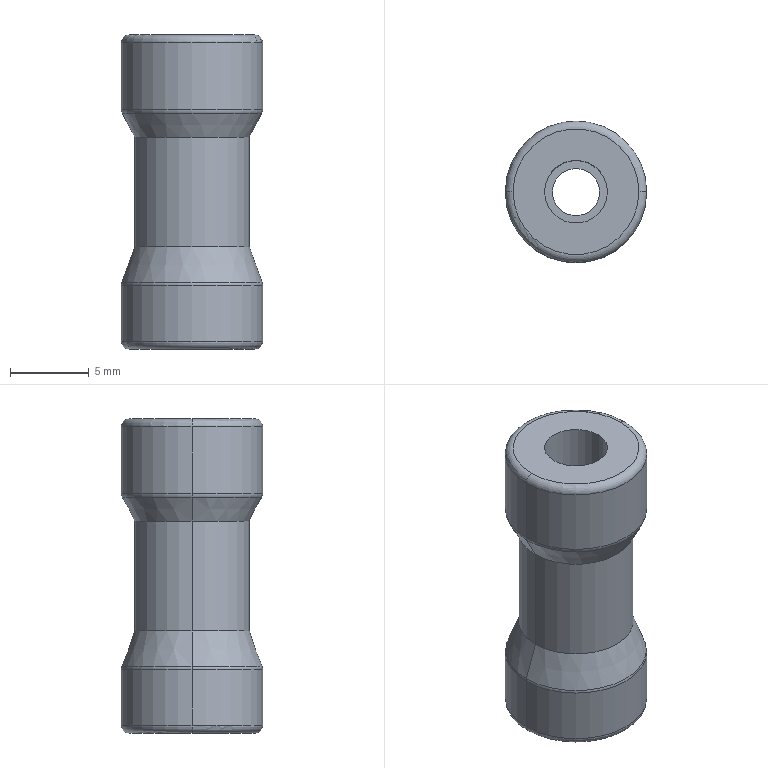Part | STEP file | Brass coupling 3-4 | 1 solid | 25 faces | box 9 x 9 x 20 mm | volume 848.219 mm3 | cylinder 10 | torus 8 | cone 4 | plane 3 | commonest cylinder face diameters 9 x4 3 x2 4 x2 7.3 x2
STEP:
#1=CARTESIAN_POINT('',(0.,0.,0.));
#2=DIRECTION('',(0.,0.,1.));
#3=DIRECTION('',(1.,0.,0.));
#4=AXIS2_PLACEMENT_3D('',#1,#2,#3);
#5=CARTESIAN_POINT('',(-1.5,0.,-2.344));
#6=VERTEX_POINT('',#5);
#7=CARTESIAN_POINT('',(-1.5,0.,-7.344));
#8=VERTEX_POINT('',#7);
#9=CARTESIAN_POINT('',(-1.5,0.,-2.344));
#10=DIRECTION('',(0.,0.,-1.));
#11=VECTOR('',#10,1.);
#12=LINE('',#9,#11);
#13=CARTESIAN_POINT('',(0.,0.,-2.344));
#14=DIRECTION('',(0.,0.,-1.));
#15=DIRECTION('',(-1.,0.,0.));
#16=AXIS2_PLACEMENT_3D('',#13,#14,#15);
#17=CYLINDRICAL_SURFACE('',#16,1.5);
#18=CARTESIAN_POINT('',(6.283,0.));
#19=DIRECTION('',(0.,1.));
#20=VECTOR('',#19,1.);
#21=LINE('',#18,#20);
#22=(GEOMETRIC_REPRESENTATION_CONTEXT(2)PARAMETRIC_REPRESENTATION_CONTEXT()REPRESENTATION_CONTEXT('',''));
#23=DEFINITIONAL_REPRESENTATION('',(#21),#22);
#24=PCURVE('',#17,#23);
#25=CARTESIAN_POINT('',(0.,0.,-2.344));
#26=DIRECTION('',(0.,0.,-1.));
#27=DIRECTION('',(-1.,0.,0.));
#28=AXIS2_PLACEMENT_3D('',#25,#26,#27);
#29=CYLINDRICAL_SURFACE('',#28,1.5);
#30=CARTESIAN_POINT('',(0.,0.));
#31=DIRECTION('',(0.,1.));
#32=VECTOR('',#31,1.);
#33=LINE('',#30,#32);
#34=(GEOMETRIC_REPRESENTATION_CONTEXT(2)PARAMETRIC_REPRESENTATION_CONTEXT()REPRESENTATION_CONTEXT('',''));
#35=DEFINITIONAL_REPRESENTATION('',(#33),#34);
#36=PCURVE('',#29,#35);
#37=SURFACE_CURVE('',#12,(#24,#36),.PCURVE_S1.);
#38=EDGE_CURVE('',#6,#8,#37,.T.);
#39=ORIENTED_EDGE('',*,*,#38,.T.);
#40=CARTESIAN_POINT('',(1.5,0.,-7.344));
#41=VERTEX_POINT('',#40);
#42=CARTESIAN_POINT('',(0.,0.,-7.344));
#43=DIRECTION('',(0.,0.,-1.));
#44=DIRECTION('',(-1.,0.,0.));
#45=AXIS2_PLACEMENT_3D('',#42,#43,#44);
#46=CIRCLE('',#45,1.5);
#47=CARTESIAN_POINT('',(0.,5.));
#48=DIRECTION('',(1.,0.));
#49=VECTOR('',#48,1.);
#50=LINE('',#47,#49);
#51=(GEOMETRIC_REPRESENTATION_CONTEXT(2)PARAMETRIC_REPRESENTATION_CONTEXT()REPRESENTATION_CONTEXT('',''));
#52=DEFINITIONAL_REPRESENTATION('',(#50),#51);
#53=PCURVE('',#17,#52);
#54=CARTESIAN_POINT('',(4.5,0.,-7.344));
#55=DIRECTION('',(0.,0.,-1.));
#56=DIRECTION('',(-1.,0.,0.));
#57=AXIS2_PLACEMENT_3D('',#54,#55,#56);
#58=PLANE('',#57);
#59=CARTESIAN_POINT('',(4.5,0.));
#60=DIRECTION('',(1.,0.));
#61=AXIS2_PLACEMENT_2D('',#59,#60);
#62=CIRCLE('',#61,1.5);
#63=(GEOMETRIC_REPRESENTATION_CONTEXT(2)PARAMETRIC_REPRESENTATION_CONTEXT()REPRESENTATION_CONTEXT('',''));
#64=DEFINITIONAL_REPRESENTATION('',(#62),#63);
#65=PCURVE('',#58,#64);
#66=SURFACE_CURVE('',#46,(#53,#65),.PCURVE_S1.);
#67=EDGE_CURVE('',#41,#8,#66,.T.);
#68=ORIENTED_EDGE('',*,*,#67,.F.);
#69=CARTESIAN_POINT('',(1.5,0.,-2.344));
#70=VERTEX_POINT('',#69);
#71=CARTESIAN_POINT('',(1.5,0.,-2.344));
#72=DIRECTION('',(0.,0.,-1.));
#73=VECTOR('',#72,1.);
#74=LINE('',#71,#73);
#75=CARTESIAN_POINT('',(3.142,0.));
#76=DIRECTION('',(0.,1.));
#77=VECTOR('',#76,1.);
#78=LINE('',#75,#77);
#79=(GEOMETRIC_REPRESENTATION_CONTEXT(2)PARAMETRIC_REPRESENTATION_CONTEXT()REPRESENTATION_CONTEXT('',''));
#80=DEFINITIONAL_REPRESENTATION('',(#78),#79);
#81=PCURVE('',#17,#80);
#82=CARTESIAN_POINT('',(3.142,0.));
#83=DIRECTION('',(0.,1.));
#84=VECTOR('',#83,1.);
#85=LINE('',#82,#84);
#86=(GEOMETRIC_REPRESENTATION_CONTEXT(2)PARAMETRIC_REPRESENTATION_CONTEXT()REPRESENTATION_CONTEXT('',''));
#87=DEFINITIONAL_REPRESENTATION('',(#85),#86);
#88=PCURVE('',#29,#87);
#89=SURFACE_CURVE('',#74,(#81,#88),.PCURVE_S1.);
#90=EDGE_CURVE('',#70,#41,#89,.T.);
#91=ORIENTED_EDGE('',*,*,#90,.F.);
#92=CARTESIAN_POINT('',(0.,0.,-2.344));
#93=DIRECTION('',(0.,0.,-1.));
#94=DIRECTION('',(-1.,0.,0.));
#95=AXIS2_PLACEMENT_3D('',#92,#93,#94);
#96=CIRCLE('',#95,1.5);
#97=CARTESIAN_POINT('',(0.,0.));
#98=DIRECTION('',(1.,0.));
#99=VECTOR('',#98,1.);
#100=LINE('',#97,#99);
#101=(GEOMETRIC_REPRESENTATION_CONTEXT(2)PARAMETRIC_REPRESENTATION_CONTEXT()REPRESENTATION_CONTEXT('',''));
#102=DEFINITIONAL_REPRESENTATION('',(#100),#101);
#103=PCURVE('',#17,#102);
#104=CARTESIAN_POINT('',(0.,0.,-2.344));
#105=DIRECTION('',(0.,0.,-1.));
#106=DIRECTION('',(-1.,0.,0.));
#107=AXIS2_PLACEMENT_3D('',#104,#105,#106);
#108=PLANE('',#107);
#109=CARTESIAN_POINT('',(0.,0.));
#110=DIRECTION('',(1.,0.));
#111=AXIS2_PLACEMENT_2D('',#109,#110);
#112=CIRCLE('',#111,1.5);
#113=(GEOMETRIC_REPRESENTATION_CONTEXT(2)PARAMETRIC_REPRESENTATION_CONTEXT()REPRESENTATION_CONTEXT('',''));
#114=DEFINITIONAL_REPRESENTATION('',(#112),#113);
#115=PCURVE('',#108,#114);
#116=SURFACE_CURVE('',#96,(#103,#115),.PCURVE_S1.);
#117=EDGE_CURVE('',#70,#6,#116,.T.);
#118=ORIENTED_EDGE('',*,*,#117,.T.);
#119=EDGE_LOOP('',(#39,#68,#91,#118));
#120=FACE_BOUND('',#119,.F.);
#121=ADVANCED_FACE('',(#120),#17,.F.);
#122=CARTESIAN_POINT('',(4.5,0.,-6.844));
#123=VERTEX_POINT('',#122);
#124=CARTESIAN_POINT('',(-4.5,0.,-6.844));
#125=VERTEX_POINT('',#124);
#126=CARTESIAN_POINT('',(0.,0.,-6.844));
#127=DIRECTION('',(0.,0.,1.));
#128=DIRECTION('',(-1.,0.,0.));
#129=AXIS2_PLACEMENT_3D('',#126,#127,#128);
#130=CIRCLE('',#129,4.5);
#131=CARTESIAN_POINT('',(0.,0.,-6.844));
#132=DIRECTION('',(0.,0.,-1.));
#133=DIRECTION('',(-1.,0.,0.));
#134=AXIS2_PLACEMENT_3D('',#131,#132,#133);
#135=TOROIDAL_SURFACE('',#134,4.,0.5);
#136=CARTESIAN_POINT('',(6.283,0.));
#137=DIRECTION('',(-1.,0.));
#138=VECTOR('',#137,1.);
#139=LINE('',#136,#138);
#140=(GEOMETRIC_REPRESENTATION_CONTEXT(2)PARAMETRIC_REPRESENTATION_CONTEXT()REPRESENTATION_CONTEXT('',''));
#141=DEFINITIONAL_REPRESENTATION('',(#139),#140);
#142=PCURVE('',#135,#141);
#143=CARTESIAN_POINT('',(0.,0.,0.));
#144=DIRECTION('',(0.,0.,1.));
#145=DIRECTION('',(1.,0.,0.));
#146=AXIS2_PLACEMENT_3D('',#143,#144,#145);
#147=CYLINDRICAL_SURFACE('',#146,4.5);
#148=CARTESIAN_POINT('',(-3.142,-6.844));
#149=DIRECTION('',(1.,0.));
#150=VECTOR('',#149,1.);
#151=LINE('',#148,#150);
#152=(GEOMETRIC_REPRESENTATION_CONTEXT(2)PARAMETRIC_REPRESENTATION_CONTEXT()REPRESENTATION_CONTEXT('',''));
#153=DEFINITIONAL_REPRESENTATION('',(#151),#152);
#154=PCURVE('',#147,#153);
#155=SURFACE_CURVE('',#130,(#142,#154),.PCURVE_S1.);
#156=EDGE_CURVE('',#123,#125,#155,.T.);
#157=ORIENTED_EDGE('',*,*,#156,.F.);
#158=CARTESIAN_POINT('',(4.,0.,-7.344));
#159=VERTEX_POINT('',#158);
#160=CARTESIAN_POINT('',(4.,0.,-6.844));
#161=DIRECTION('',(0.,1.,0.));
#162=DIRECTION('',(-1.,0.,0.));
#163=AXIS2_PLACEMENT_3D('',#160,#161,#162);
#164=CIRCLE('',#163,0.5);
#165=CARTESIAN_POINT('',(3.142,-3.142));
#166=DIRECTION('',(0.,1.));
#167=VECTOR('',#166,1.);
#168=LINE('',#165,#167);
#169=(GEOMETRIC_REPRESENTATION_CONTEXT(2)PARAMETRIC_REPRESENTATION_CONTEXT()REPRESENTATION_CONTEXT('',''));
#170=DEFINITIONAL_REPRESENTATION('',(#168),#169);
#171=PCURVE('',#135,#170);
#172=CARTESIAN_POINT('',(0.,0.,-6.844));
#173=DIRECTION('',(0.,0.,-1.));
#174=DIRECTION('',(-1.,0.,0.));
#175=AXIS2_PLACEMENT_3D('',#172,#173,#174);
#176=TOROIDAL_SURFACE('',#175,4.,0.5);
#177=CARTESIAN_POINT('',(3.142,-3.142));
#178=DIRECTION('',(0.,1.));
#179=VECTOR('',#178,1.);
#180=LINE('',#177,#179);
#181=(GEOMETRIC_REPRESENTATION_CONTEXT(2)PARAMETRIC_REPRESENTATION_CONTEXT()REPRESENTATION_CONTEXT('',''));
#182=DEFINITIONAL_REPRESENTATION('',(#180),#181);
#183=PCURVE('',#176,#182);
#184=SURFACE_CURVE('',#164,(#171,#183),.PCURVE_S1.);
#185=EDGE_CURVE('',#123,#159,#184,.T.);
#186=ORIENTED_EDGE('',*,*,#185,.T.);
#187=CARTESIAN_POINT('',(-4.,0.,-7.344));
#188=VERTEX_POINT('',#187);
#189=CARTESIAN_POINT('',(0.,0.,-7.344));
#190=DIRECTION('',(0.,0.,-1.));
#191=DIRECTION('',(-1.,0.,0.));
#192=AXIS2_PLACEMENT_3D('',#189,#190,#191);
#193=CIRCLE('',#192,4.);
#194=CARTESIAN_POINT('',(0.,1.571));
#195=DIRECTION('',(1.,0.));
#196=VECTOR('',#195,1.);
#197=LINE('',#194,#196);
#198=(GEOMETRIC_REPRESENTATION_CONTEXT(2)PARAMETRIC_REPRESENTATION_CONTEXT()REPRESENTATION_CONTEXT('',''));
#199=DEFINITIONAL_REPRESENTATION('',(#197),#198);
#200=PCURVE('',#135,#199);
#201=CARTESIAN_POINT('',(4.5,0.));
#202=DIRECTION('',(1.,0.));
#203=AXIS2_PLACEMENT_2D('',#201,#202);
#204=CIRCLE('',#203,4.);
#205=(GEOMETRIC_REPRESENTATION_CONTEXT(2)PARAMETRIC_REPRESENTATION_CONTEXT()REPRESENTATION_CONTEXT('',''));
#206=DEFINITIONAL_REPRESENTATION('',(#204),#205);
#207=PCURVE('',#58,#206);
#208=SURFACE_CURVE('',#193,(#200,#207),.PCURVE_S1.);
#209=EDGE_CURVE('',#188,#159,#208,.T.);
#210=ORIENTED_EDGE('',*,*,#209,.F.);
#211=CARTESIAN_POINT('',(-4.,0.,-6.844));
#212=DIRECTION('',(0.,-1.,0.));
#213=DIRECTION('',(0.,0.,-1.));
#214=AXIS2_PLACEMENT_3D('',#211,#212,#213);
#215=CIRCLE('',#214,0.5);
#216=CARTESIAN_POINT('',(0.,-4.712));
#217=DIRECTION('',(0.,1.));
#218=VECTOR('',#217,1.);
#219=LINE('',#216,#218);
#220=(GEOMETRIC_REPRESENTATION_CONTEXT(2)PARAMETRIC_REPRESENTATION_CONTEXT()REPRESENTATION_CONTEXT('',''));
#221=DEFINITIONAL_REPRESENTATION('',(#219),#220);
#222=PCURVE('',#135,#221);
#223=CARTESIAN_POINT('',(6.283,-4.712));
#224=DIRECTION('',(0.,1.));
#225=VECTOR('',#224,1.);
#226=LINE('',#223,#225);
#227=(GEOMETRIC_REPRESENTATION_CONTEXT(2)PARAMETRIC_REPRESENTATION_CONTEXT()REPRESENTATION_CONTEXT('',''));
#228=DEFINITIONAL_REPRESENTATION('',(#226),#227);
#229=PCURVE('',#176,#228);
#230=SURFACE_CURVE('',#215,(#222,#229),.PCURVE_S1.);
#231=EDGE_CURVE('',#125,#188,#230,.T.);
#232=ORIENTED_EDGE('',*,*,#231,.F.);
#233=EDGE_LOOP('',(#157,#186,#210,#232));
#234=FACE_BOUND('',#233,.T.);
#235=ADVANCED_FACE('',(#234),#135,.T.);
#236=CARTESIAN_POINT('',(4.47,0.,-3.119));
#237=VERTEX_POINT('',#236);
#238=CARTESIAN_POINT('',(-4.47,0.,-3.119));
#239=VERTEX_POINT('',#238);
#240=CARTESIAN_POINT('',(0.,0.,-3.119));
#241=DIRECTION('',(0.,0.,1.));
#242=DIRECTION('',(1.,0.,0.));
#243=AXIS2_PLACEMENT_3D('',#240,#241,#242);
#244=CIRCLE('',#243,4.47);
#245=CARTESIAN_POINT('',(0.,0.,-3.289));
#246=DIRECTION('',(0.,0.,-1.));
#247=DIRECTION('',(-1.,0.,0.));
#248=AXIS2_PLACEMENT_3D('',#245,#246,#247);
#249=TOROIDAL_SURFACE('',#248,4.,0.5);
#250=CARTESIAN_POINT('',(3.142,5.937));
#251=DIRECTION('',(-1.,0.));
#252=VECTOR('',#251,1.);
#253=LINE('',#250,#252);
#254=(GEOMETRIC_REPRESENTATION_CONTEXT(2)PARAMETRIC_REPRESENTATION_CONTEXT()REPRESENTATION_CONTEXT('',''));
#255=DEFINITIONAL_REPRESENTATION('',(#253),#254);
#256=PCURVE('',#249,#255);
#257=CARTESIAN_POINT('',(0.,0.,-0.844));
#258=DIRECTION('',(0.,0.,-1.));
#259=DIRECTION('',(-1.,0.,0.));
#260=AXIS2_PLACEMENT_3D('',#257,#258,#259);
#261=CONICAL_SURFACE('',#260,3.65,0.3461);
#262=CARTESIAN_POINT('',(3.142,2.275));
#263=DIRECTION('',(-1.,0.));
#264=VECTOR('',#263,1.);
#265=LINE('',#262,#264);
#266=(GEOMETRIC_REPRESENTATION_CONTEXT(2)PARAMETRIC_REPRESENTATION_CONTEXT()REPRESENTATION_CONTEXT('',''));
#267=DEFINITIONAL_REPRESENTATION('',(#265),#266);
#268=PCURVE('',#261,#267);
#269=SURFACE_CURVE('',#244,(#256,#268),.PCURVE_S1.);
#270=EDGE_CURVE('',#237,#239,#269,.T.);
#271=ORIENTED_EDGE('',*,*,#270,.F.);
#272=CARTESIAN_POINT('',(4.5,0.,-3.289));
#273=VERTEX_POINT('',#272);
#274=CARTESIAN_POINT('',(4.,0.,-3.289));
#275=DIRECTION('',(0.,1.,0.));
#276=DIRECTION('',(-1.,0.,0.));
#277=AXIS2_PLACEMENT_3D('',#274,#275,#276);
#278=CIRCLE('',#277,0.5);
#279=CARTESIAN_POINT('',(3.142,3.142));
#280=DIRECTION('',(0.,1.));
#281=VECTOR('',#280,1.);
#282=LINE('',#279,#281);
#283=(GEOMETRIC_REPRESENTATION_CONTEXT(2)PARAMETRIC_REPRESENTATION_CONTEXT()REPRESENTATION_CONTEXT('',''));
#284=DEFINITIONAL_REPRESENTATION('',(#282),#283);
#285=PCURVE('',#249,#284);
#286=CARTESIAN_POINT('',(0.,0.,-3.289));
#287=DIRECTION('',(0.,0.,-1.));
#288=DIRECTION('',(-1.,0.,0.));
#289=AXIS2_PLACEMENT_3D('',#286,#287,#288);
#290=TOROIDAL_SURFACE('',#289,4.,0.5);
#291=CARTESIAN_POINT('',(3.142,3.142));
#292=DIRECTION('',(0.,1.));
#293=VECTOR('',#292,1.);
#294=LINE('',#291,#293);
#295=(GEOMETRIC_REPRESENTATION_CONTEXT(2)PARAMETRIC_REPRESENTATION_CONTEXT()REPRESENTATION_CONTEXT('',''));
#296=DEFINITIONAL_REPRESENTATION('',(#294),#295);
#297=PCURVE('',#290,#296);
#298=SURFACE_CURVE('',#278,(#285,#297),.PCURVE_S1.);
#299=EDGE_CURVE('',#237,#273,#298,.T.);
#300=ORIENTED_EDGE('',*,*,#299,.T.);
#301=CARTESIAN_POINT('',(-4.5,0.,-3.289));
#302=VERTEX_POINT('',#301);
#303=CARTESIAN_POINT('',(0.,0.,-3.289));
#304=DIRECTION('',(0.,0.,-1.));
#305=DIRECTION('',(-1.,0.,0.));
#306=AXIS2_PLACEMENT_3D('',#303,#304,#305);
#307=CIRCLE('',#306,4.5);
#308=CARTESIAN_POINT('',(0.,6.283));
#309=DIRECTION('',(1.,0.));
#310=VECTOR('',#309,1.);
#311=LINE('',#308,#310);
#312=(GEOMETRIC_REPRESENTATION_CONTEXT(2)PARAMETRIC_REPRESENTATION_CONTEXT()REPRESENTATION_CONTEXT('',''));
#313=DEFINITIONAL_REPRESENTATION('',(#311),#312);
#314=PCURVE('',#249,#313);
#315=CARTESIAN_POINT('',(3.142,-3.289));
#316=DIRECTION('',(-1.,0.));
#317=VECTOR('',#316,1.);
#318=LINE('',#315,#317);
#319=(GEOMETRIC_REPRESENTATION_CONTEXT(2)PARAMETRIC_REPRESENTATION_CONTEXT()REPRESENTATION_CONTEXT('',''));
#320=DEFINITIONAL_REPRESENTATION('',(#318),#319);
#321=PCURVE('',#147,#320);
#322=SURFACE_CURVE('',#307,(#314,#321),.PCURVE_S1.);
#323=EDGE_CURVE('',#302,#273,#322,.T.);
#324=ORIENTED_EDGE('',*,*,#323,.F.);
#325=CARTESIAN_POINT('',(-4.,0.,-3.289));
#326=DIRECTION('',(0.,-1.,0.));
#327=DIRECTION('',(0.,0.,-1.));
#328=AXIS2_PLACEMENT_3D('',#325,#326,#327);
#329=CIRCLE('',#328,0.5);
#330=CARTESIAN_POINT('',(0.,1.571));
#331=DIRECTION('',(0.,1.));
#332=VECTOR('',#331,1.);
#333=LINE('',#330,#332);
#334=(GEOMETRIC_REPRESENTATION_CONTEXT(2)PARAMETRIC_REPRESENTATION_CONTEXT()REPRESENTATION_CONTEXT('',''));
#335=DEFINITIONAL_REPRESENTATION('',(#333),#334);
#336=PCURVE('',#249,#335);
#337=CARTESIAN_POINT('',(6.283,1.571));
#338=DIRECTION('',(0.,1.));
#339=VECTOR('',#338,1.);
#340=LINE('',#337,#339);
#341=(GEOMETRIC_REPRESENTATION_CONTEXT(2)PARAMETRIC_REPRESENTATION_CONTEXT()REPRESENTATION_CONTEXT('',''));
#342=DEFINITIONAL_REPRESENTATION('',(#340),#341);
#343=PCURVE('',#290,#342);
#344=SURFACE_CURVE('',#329,(#336,#343),.PCURVE_S1.);
#345=EDGE_CURVE('',#239,#302,#344,.T.);
#346=ORIENTED_EDGE('',*,*,#345,.F.);
#347=EDGE_LOOP('',(#271,#300,#324,#346));
#348=FACE_BOUND('',#347,.T.);
#349=ADVANCED_FACE('',(#348),#249,.T.);
#350=CARTESIAN_POINT('',(4.5,0.,7.912));
#351=VERTEX_POINT('',#350);
#352=CARTESIAN_POINT('',(-4.5,0.,7.912));
#353=VERTEX_POINT('',#352);
#354=CARTESIAN_POINT('',(0.,0.,7.912));
#355=DIRECTION('',(0.,0.,1.));
#356=DIRECTION('',(-1.,0.,0.));
#357=AXIS2_PLACEMENT_3D('',#354,#355,#356);
#358=CIRCLE('',#357,4.5);
#359=CARTESIAN_POINT('',(0.,0.,7.912));
#360=DIRECTION('',(0.,0.,-1.));
#361=DIRECTION('',(-1.,0.,0.));
#362=AXIS2_PLACEMENT_3D('',#359,#360,#361);
#363=TOROIDAL_SURFACE('',#362,4.,0.5);
#364=CARTESIAN_POINT('',(6.283,0.));
#365=DIRECTION('',(-1.,0.));
#366=VECTOR('',#365,1.);
#367=LINE('',#364,#366);
#368=(GEOMETRIC_REPRESENTATION_CONTEXT(2)PARAMETRIC_REPRESENTATION_CONTEXT()REPRESENTATION_CONTEXT('',''));
#369=DEFINITIONAL_REPRESENTATION('',(#367),#368);
#370=PCURVE('',#363,#369);
#371=CARTESIAN_POINT('',(0.,0.,0.));
#372=DIRECTION('',(0.,0.,1.));
#373=DIRECTION('',(1.,0.,0.));
#374=AXIS2_PLACEMENT_3D('',#371,#372,#373);
#375=CYLINDRICAL_SURFACE('',#374,4.5);
#376=CARTESIAN_POINT('',(-3.142,7.912));
#377=DIRECTION('',(1.,0.));
#378=VECTOR('',#377,1.);
#379=LINE('',#376,#378);
#380=(GEOMETRIC_REPRESENTATION_CONTEXT(2)PARAMETRIC_REPRESENTATION_CONTEXT()REPRESENTATION_CONTEXT('',''));
#381=DEFINITIONAL_REPRESENTATION('',(#379),#380);
#382=PCURVE('',#375,#381);
#383=SURFACE_CURVE('',#358,(#370,#382),.PCURVE_S1.);
#384=EDGE_CURVE('',#351,#353,#383,.T.);
#385=ORIENTED_EDGE('',*,*,#384,.F.);
#386=CARTESIAN_POINT('',(4.444,0.,7.681));
#387=VERTEX_POINT('',#386);
#388=CARTESIAN_POINT('',(4.,0.,7.912));
#389=DIRECTION('',(0.,1.,0.));
#390=DIRECTION('',(-1.,0.,0.));
#391=AXIS2_PLACEMENT_3D('',#388,#389,#390);
#392=CIRCLE('',#391,0.5);
#393=CARTESIAN_POINT('',(3.142,-3.142));
#394=DIRECTION('',(0.,1.));
#395=VECTOR('',#394,1.);
#396=LINE('',#393,#395);
#397=(GEOMETRIC_REPRESENTATION_CONTEXT(2)PARAMETRIC_REPRESENTATION_CONTEXT()REPRESENTATION_CONTEXT('',''));
#398=DEFINITIONAL_REPRESENTATION('',(#396),#397);
#399=PCURVE('',#363,#398);
#400=CARTESIAN_POINT('',(0.,0.,7.912));
#401=DIRECTION('',(0.,0.,-1.));
#402=DIRECTION('',(-1.,0.,0.));
#403=AXIS2_PLACEMENT_3D('',#400,#401,#402);
#404=TOROIDAL_SURFACE('',#403,4.,0.5);
#405=CARTESIAN_POINT('',(3.142,-3.142));
#406=DIRECTION('',(0.,1.));
#407=VECTOR('',#406,1.);
#408=LINE('',#405,#407);
#409=(GEOMETRIC_REPRESENTATION_CONTEXT(2)PARAMETRIC_REPRESENTATION_CONTEXT()REPRESENTATION_CONTEXT('',''));
#410=DEFINITIONAL_REPRESENTATION('',(#408),#409);
#411=PCURVE('',#404,#410);
#412=SURFACE_CURVE('',#392,(#399,#411),.PCURVE_S1.);
#413=EDGE_CURVE('',#351,#387,#412,.T.);
#414=ORIENTED_EDGE('',*,*,#413,.T.);
#415=CARTESIAN_POINT('',(-4.444,0.,7.681));
#416=VERTEX_POINT('',#415);
#417=CARTESIAN_POINT('',(0.,0.,7.681));
#418=DIRECTION('',(0.,0.,-1.));
#419=DIRECTION('',(-1.,0.,0.));
#420=AXIS2_PLACEMENT_3D('',#417,#418,#419);
#421=CIRCLE('',#420,4.444);
#422=CARTESIAN_POINT('',(0.,0.4797));
#423=DIRECTION('',(1.,0.));
#424=VECTOR('',#423,1.);
#425=LINE('',#422,#424);
#426=(GEOMETRIC_REPRESENTATION_CONTEXT(2)PARAMETRIC_REPRESENTATION_CONTEXT()REPRESENTATION_CONTEXT('',''));
#427=DEFINITIONAL_REPRESENTATION('',(#425),#426);
#428=PCURVE('',#363,#427);
#429=CARTESIAN_POINT('',(0.,0.,7.79));
#430=DIRECTION('',(0.,0.,1.));
#431=DIRECTION('',(1.,0.,0.));
#432=AXIS2_PLACEMENT_3D('',#429,#430,#431);
#433=CONICAL_SURFACE('',#432,4.5,0.4797);
#434=CARTESIAN_POINT('',(3.142,-0.1085));
#435=DIRECTION('',(-1.,0.));
#436=VECTOR('',#435,1.);
#437=LINE('',#434,#436);
#438=(GEOMETRIC_REPRESENTATION_CONTEXT(2)PARAMETRIC_REPRESENTATION_CONTEXT()REPRESENTATION_CONTEXT('',''));
#439=DEFINITIONAL_REPRESENTATION('',(#437),#438);
#440=PCURVE('',#433,#439);
#441=SURFACE_CURVE('',#421,(#428,#440),.PCURVE_S1.);
#442=EDGE_CURVE('',#416,#387,#441,.T.);
#443=ORIENTED_EDGE('',*,*,#442,.F.);
#444=CARTESIAN_POINT('',(-4.,0.,7.912));
#445=DIRECTION('',(0.,-1.,0.));
#446=DIRECTION('',(0.,0.,-1.));
#447=AXIS2_PLACEMENT_3D('',#444,#445,#446);
#448=CIRCLE('',#447,0.5);
#449=CARTESIAN_POINT('',(0.,-4.712));
#450=DIRECTION('',(0.,1.));
#451=VECTOR('',#450,1.);
#452=LINE('',#449,#451);
#453=(GEOMETRIC_REPRESENTATION_CONTEXT(2)PARAMETRIC_REPRESENTATION_CONTEXT()REPRESENTATION_CONTEXT('',''));
#454=DEFINITIONAL_REPRESENTATION('',(#452),#453);
#455=PCURVE('',#363,#454);
#456=CARTESIAN_POINT('',(6.283,-4.712));
#457=DIRECTION('',(0.,1.));
#458=VECTOR('',#457,1.);
#459=LINE('',#456,#458);
#460=(GEOMETRIC_REPRESENTATION_CONTEXT(2)PARAMETRIC_REPRESENTATION_CONTEXT()REPRESENTATION_CONTEXT('',''));
#461=DEFINITIONAL_REPRESENTATION('',(#459),#460);
#462=PCURVE('',#404,#461);
#463=SURFACE_CURVE('',#448,(#455,#462),.PCURVE_S1.);
#464=EDGE_CURVE('',#353,#416,#463,.T.);
#465=ORIENTED_EDGE('',*,*,#464,.F.);
#466=EDGE_LOOP('',(#385,#414,#443,#465));
#467=FACE_BOUND('',#466,.T.);
#468=ADVANCED_FACE('',(#467),#363,.T.);
#469=CARTESIAN_POINT('',(-4.5,0.,12.156));
#470=VERTEX_POINT('',#469);
#471=CARTESIAN_POINT('',(4.5,0.,12.156));
#472=VERTEX_POINT('',#471);
#473=CARTESIAN_POINT('',(0.,0.,12.156));
#474=DIRECTION('',(0.,0.,-1.));
#475=DIRECTION('',(1.,0.,0.));
#476=AXIS2_PLACEMENT_3D('',#473,#474,#475);
#477=CIRCLE('',#476,4.5);
#478=CARTESIAN_POINT('',(0.,0.,12.156));
#479=DIRECTION('',(0.,0.,1.));
#480=DIRECTION('',(1.,0.,0.));
#481=AXIS2_PLACEMENT_3D('',#478,#479,#480);
#482=TOROIDAL_SURFACE('',#481,4.,0.5);
#483=CARTESIAN_POINT('',(6.283,0.));
#484=DIRECTION('',(-1.,0.));
#485=VECTOR('',#484,1.);
#486=LINE('',#483,#485);
#487=(GEOMETRIC_REPRESENTATION_CONTEXT(2)PARAMETRIC_REPRESENTATION_CONTEXT()REPRESENTATION_CONTEXT('',''));
#488=DEFINITIONAL_REPRESENTATION('',(#486),#487);
#489=PCURVE('',#482,#488);
#490=CARTESIAN_POINT('',(6.283,12.156));
#491=DIRECTION('',(-1.,0.));
#492=VECTOR('',#491,1.);
#493=LINE('',#490,#492);
#494=(GEOMETRIC_REPRESENTATION_CONTEXT(2)PARAMETRIC_REPRESENTATION_CONTEXT()REPRESENTATION_CONTEXT('',''));
#495=DEFINITIONAL_REPRESENTATION('',(#493),#494);
#496=PCURVE('',#375,#495);
#497=SURFACE_CURVE('',#477,(#489,#496),.PCURVE_S1.);
#498=EDGE_CURVE('',#470,#472,#497,.T.);
#499=ORIENTED_EDGE('',*,*,#498,.F.);
#500=CARTESIAN_POINT('',(-4.,0.,12.656));
#501=VERTEX_POINT('',#500);
#502=CARTESIAN_POINT('',(-4.,0.,12.156));
#503=DIRECTION('',(0.,1.,0.));
#504=DIRECTION('',(-1.,0.,0.));
#505=AXIS2_PLACEMENT_3D('',#502,#503,#504);
#506=CIRCLE('',#505,0.5);
#507=CARTESIAN_POINT('',(3.142,0.));
#508=DIRECTION('',(0.,1.));
#509=VECTOR('',#508,1.);
#510=LINE('',#507,#509);
#511=(GEOMETRIC_REPRESENTATION_CONTEXT(2)PARAMETRIC_REPRESENTATION_CONTEXT()REPRESENTATION_CONTEXT('',''));
#512=DEFINITIONAL_REPRESENTATION('',(#510),#511);
#513=PCURVE('',#482,#512);
#514=CARTESIAN_POINT('',(0.,0.,12.156));
#515=DIRECTION('',(0.,0.,1.));
#516=DIRECTION('',(1.,0.,0.));
#517=AXIS2_PLACEMENT_3D('',#514,#515,#516);
#518=TOROIDAL_SURFACE('',#517,4.,0.5);
#519=CARTESIAN_POINT('',(3.142,0.));
#520=DIRECTION('',(0.,1.));
#521=VECTOR('',#520,1.);
#522=LINE('',#519,#521);
#523=(GEOMETRIC_REPRESENTATION_CONTEXT(2)PARAMETRIC_REPRESENTATION_CONTEXT()REPRESENTATION_CONTEXT('',''));
#524=DEFINITIONAL_REPRESENTATION('',(#522),#523);
#525=PCURVE('',#518,#524);
#526=SURFACE_CURVE('',#506,(#513,#525),.PCURVE_S1.);
#527=EDGE_CURVE('',#470,#501,#526,.T.);
#528=ORIENTED_EDGE('',*,*,#527,.T.);
#529=CARTESIAN_POINT('',(4.,0.,12.656));
#530=VERTEX_POINT('',#529);
#531=CARTESIAN_POINT('',(0.,0.,12.656));
#532=DIRECTION('',(0.,0.,1.));
#533=DIRECTION('',(1.,0.,0.));
#534=AXIS2_PLACEMENT_3D('',#531,#532,#533);
#535=CIRCLE('',#534,4.);
#536=CARTESIAN_POINT('',(0.,1.571));
#537=DIRECTION('',(1.,0.));
#538=VECTOR('',#537,1.);
#539=LINE('',#536,#538);
#540=(GEOMETRIC_REPRESENTATION_CONTEXT(2)PARAMETRIC_REPRESENTATION_CONTEXT()REPRESENTATION_CONTEXT('',''));
#541=DEFINITIONAL_REPRESENTATION('',(#539),#540);
#542=PCURVE('',#482,#541);
#543=CARTESIAN_POINT('',(1.052,0.,12.656));
#544=DIRECTION('',(0.,0.,1.));
#545=DIRECTION('',(1.,0.,0.));
#546=AXIS2_PLACEMENT_3D('',#543,#544,#545);
#547=PLANE('',#546);
#548=CARTESIAN_POINT('',(-1.052,0.));
#549=DIRECTION('',(1.,0.));
#550=AXIS2_PLACEMENT_2D('',#548,#549);
#551=CIRCLE('',#550,4.);
#552=(GEOMETRIC_REPRESENTATION_CONTEXT(2)PARAMETRIC_REPRESENTATION_CONTEXT()REPRESENTATION_CONTEXT('',''));
#553=DEFINITIONAL_REPRESENTATION('',(#551),#552);
#554=PCURVE('',#547,#553);
#555=SURFACE_CURVE('',#535,(#542,#554),.PCURVE_S1.);
#556=EDGE_CURVE('',#530,#501,#555,.T.);
#557=ORIENTED_EDGE('',*,*,#556,.F.);
#558=CARTESIAN_POINT('',(4.,0.,12.156));
#559=DIRECTION('',(0.,-1.,0.));
#560=DIRECTION('',(0.,0.,-1.));
#561=AXIS2_PLACEMENT_3D('',#558,#559,#560);
#562=CIRCLE('',#561,0.5);
#563=CARTESIAN_POINT('',(0.,-1.571));
#564=DIRECTION('',(0.,1.));
#565=VECTOR('',#564,1.);
#566=LINE('',#563,#565);
#567=(GEOMETRIC_REPRESENTATION_CONTEXT(2)PARAMETRIC_REPRESENTATION_CONTEXT()REPRESENTATION_CONTEXT('',''));
#568=DEFINITIONAL_REPRESENTATION('',(#566),#567);
#569=PCURVE('',#482,#568);
#570=CARTESIAN_POINT('',(6.283,-1.571));
#571=DIRECTION('',(0.,1.));
#572=VECTOR('',#571,1.);
#573=LINE('',#570,#572);
#574=(GEOMETRIC_REPRESENTATION_CONTEXT(2)PARAMETRIC_REPRESENTATION_CONTEXT()REPRESENTATION_CONTEXT('',''));
#575=DEFINITIONAL_REPRESENTATION('',(#573),#574);
#576=PCURVE('',#518,#575);
#577=SURFACE_CURVE('',#562,(#569,#576),.PCURVE_S1.);
#578=EDGE_CURVE('',#472,#530,#577,.T.);
#579=ORIENTED_EDGE('',*,*,#578,.F.);
#580=EDGE_LOOP('',(#499,#528,#557,#579));
#581=FACE_BOUND('',#580,.T.);
#582=ADVANCED_FACE('',(#581),#482,.T.);
#583=ORIENTED_EDGE('',*,*,#156,.T.);
#584=CARTESIAN_POINT('',(-4.5,0.,0.));
#585=DIRECTION('',(0.,0.,1.));
#586=VECTOR('',#585,1.);
#587=LINE('',#584,#586);
#588=CARTESIAN_POINT('',(3.142,0.));
#589=DIRECTION('',(0.,1.));
#590=VECTOR('',#589,1.);
#591=LINE('',#588,#590);
#592=(GEOMETRIC_REPRESENTATION_CONTEXT(2)PARAMETRIC_REPRESENTATION_CONTEXT()REPRESENTATION_CONTEXT('',''));
#593=DEFINITIONAL_REPRESENTATION('',(#591),#592);
#594=PCURVE('',#147,#593);
#595=CARTESIAN_POINT('',(0.,0.,0.));
#596=DIRECTION('',(0.,0.,1.));
#597=DIRECTION('',(1.,0.,0.));
#598=AXIS2_PLACEMENT_3D('',#595,#596,#597);
#599=CYLINDRICAL_SURFACE('',#598,4.5);
#600=CARTESIAN_POINT('',(3.142,0.));
#601=DIRECTION('',(0.,1.));
#602=VECTOR('',#601,1.);
#603=LINE('',#600,#602);
#604=(GEOMETRIC_REPRESENTATION_CONTEXT(2)PARAMETRIC_REPRESENTATION_CONTEXT()REPRESENTATION_CONTEXT('',''));
#605=DEFINITIONAL_REPRESENTATION('',(#603),#604);
#606=PCURVE('',#599,#605);
#607=SURFACE_CURVE('',#587,(#594,#606),.PCURVE_S1.);
#608=EDGE_CURVE('',#125,#302,#607,.T.);
#609=ORIENTED_EDGE('',*,*,#608,.T.);
#610=ORIENTED_EDGE('',*,*,#323,.T.);
#611=CARTESIAN_POINT('',(4.5,0.,0.));
#612=DIRECTION('',(0.,0.,1.));
#613=VECTOR('',#612,1.);
#614=LINE('',#611,#613);
#615=CARTESIAN_POINT('',(0.,0.));
#616=DIRECTION('',(0.,1.));
#617=VECTOR('',#616,1.);
#618=LINE('',#615,#617);
#619=(GEOMETRIC_REPRESENTATION_CONTEXT(2)PARAMETRIC_REPRESENTATION_CONTEXT()REPRESENTATION_CONTEXT('',''));
#620=DEFINITIONAL_REPRESENTATION('',(#618),#619);
#621=PCURVE('',#147,#620);
#622=CARTESIAN_POINT('',(6.283,0.));
#623=DIRECTION('',(0.,1.));
#624=VECTOR('',#623,1.);
#625=LINE('',#622,#624);
#626=(GEOMETRIC_REPRESENTATION_CONTEXT(2)PARAMETRIC_REPRESENTATION_CONTEXT()REPRESENTATION_CONTEXT('',''));
#627=DEFINITIONAL_REPRESENTATION('',(#625),#626);
#628=PCURVE('',#599,#627);
#629=SURFACE_CURVE('',#614,(#621,#628),.PCURVE_S1.);
#630=EDGE_CURVE('',#123,#273,#629,.T.);
#631=ORIENTED_EDGE('',*,*,#630,.F.);
#632=EDGE_LOOP('',(#583,#609,#610,#631));
#633=FACE_BOUND('',#632,.T.);
#634=ADVANCED_FACE('',(#633),#147,.T.);
#635=CARTESIAN_POINT('',(3.65,0.,-0.844));
#636=VERTEX_POINT('',#635);
#637=CARTESIAN_POINT('',(-3.65,0.,-0.844));
#638=VERTEX_POINT('',#637);
#639=CARTESIAN_POINT('',(0.,0.,-0.844));
#640=DIRECTION('',(0.,0.,1.));
#641=DIRECTION('',(1.,0.,0.));
#642=AXIS2_PLACEMENT_3D('',#639,#640,#641);
#643=CIRCLE('',#642,3.65);
#644=CARTESIAN_POINT('',(3.142,0.));
#645=DIRECTION('',(-1.,0.));
#646=VECTOR('',#645,1.);
#647=LINE('',#644,#646);
#648=(GEOMETRIC_REPRESENTATION_CONTEXT(2)PARAMETRIC_REPRESENTATION_CONTEXT()REPRESENTATION_CONTEXT('',''));
#649=DEFINITIONAL_REPRESENTATION('',(#647),#648);
#650=PCURVE('',#261,#649);
#651=CARTESIAN_POINT('',(0.,0.,0.));
#652=DIRECTION('',(0.,0.,1.));
#653=DIRECTION('',(1.,0.,0.));
#654=AXIS2_PLACEMENT_3D('',#651,#652,#653);
#655=CYLINDRICAL_SURFACE('',#654,3.65);
#656=CARTESIAN_POINT('',(0.,-0.844));
#657=DIRECTION('',(1.,0.));
#658=VECTOR('',#657,1.);
#659=LINE('',#656,#658);
#660=(GEOMETRIC_REPRESENTATION_CONTEXT(2)PARAMETRIC_REPRESENTATION_CONTEXT()REPRESENTATION_CONTEXT('',''));
#661=DEFINITIONAL_REPRESENTATION('',(#659),#660);
#662=PCURVE('',#655,#661);
#663=SURFACE_CURVE('',#643,(#650,#662),.PCURVE_S1.);
#664=EDGE_CURVE('',#636,#638,#663,.T.);
#665=ORIENTED_EDGE('',*,*,#664,.F.);
#666=CARTESIAN_POINT('',(3.65,0.,-0.844));
#667=DIRECTION('',(0.3392,0.,-0.9407));
#668=VECTOR('',#667,1.);
#669=LINE('',#666,#668);
#670=CARTESIAN_POINT('',(3.142,0.));
#671=DIRECTION('',(0.,1.));
#672=VECTOR('',#671,1.);
#673=LINE('',#670,#672);
#674=(GEOMETRIC_REPRESENTATION_CONTEXT(2)PARAMETRIC_REPRESENTATION_CONTEXT()REPRESENTATION_CONTEXT('',''));
#675=DEFINITIONAL_REPRESENTATION('',(#673),#674);
#676=PCURVE('',#261,#675);
#677=CARTESIAN_POINT('',(0.,0.,-0.844));
#678=DIRECTION('',(0.,0.,-1.));
#679=DIRECTION('',(-1.,0.,0.));
#680=AXIS2_PLACEMENT_3D('',#677,#678,#679);
#681=CONICAL_SURFACE('',#680,3.65,0.3461);
#682=CARTESIAN_POINT('',(3.142,0.));
#683=DIRECTION('',(0.,1.));
#684=VECTOR('',#683,1.);
#685=LINE('',#682,#684);
#686=(GEOMETRIC_REPRESENTATION_CONTEXT(2)PARAMETRIC_REPRESENTATION_CONTEXT()REPRESENTATION_CONTEXT('',''));
#687=DEFINITIONAL_REPRESENTATION('',(#685),#686);
#688=PCURVE('',#681,#687);
#689=SURFACE_CURVE('',#669,(#676,#688),.PCURVE_S1.);
#690=EDGE_CURVE('',#636,#237,#689,.T.);
#691=ORIENTED_EDGE('',*,*,#690,.T.);
#692=ORIENTED_EDGE('',*,*,#270,.T.);
#693=CARTESIAN_POINT('',(-3.65,0.,-0.844));
#694=DIRECTION('',(-0.3392,0.,-0.9407));
#695=VECTOR('',#694,1.);
#696=LINE('',#693,#695);
#697=CARTESIAN_POINT('',(0.,0.));
#698=DIRECTION('',(0.,1.));
#699=VECTOR('',#698,1.);
#700=LINE('',#697,#699);
#701=(GEOMETRIC_REPRESENTATION_CONTEXT(2)PARAMETRIC_REPRESENTATION_CONTEXT()REPRESENTATION_CONTEXT('',''));
#702=DEFINITIONAL_REPRESENTATION('',(#700),#701);
#703=PCURVE('',#261,#702);
#704=CARTESIAN_POINT('',(6.283,0.));
#705=DIRECTION('',(0.,1.));
#706=VECTOR('',#705,1.);
#707=LINE('',#704,#706);
#708=(GEOMETRIC_REPRESENTATION_CONTEXT(2)PARAMETRIC_REPRESENTATION_CONTEXT()REPRESENTATION_CONTEXT('',''));
#709=DEFINITIONAL_REPRESENTATION('',(#707),#708);
#710=PCURVE('',#681,#709);
#711=SURFACE_CURVE('',#696,(#703,#710),.PCURVE_S1.);
#712=EDGE_CURVE('',#638,#239,#711,.T.);
#713=ORIENTED_EDGE('',*,*,#712,.F.);
#714=EDGE_LOOP('',(#665,#691,#692,#713));
#715=FACE_BOUND('',#714,.T.);
#716=ADVANCED_FACE('',(#715),#261,.T.);
#717=ORIENTED_EDGE('',*,*,#664,.T.);
#718=CARTESIAN_POINT('',(-3.65,0.,6.156));
#719=VERTEX_POINT('',#718);
#720=CARTESIAN_POINT('',(-3.65,0.,0.));
#721=DIRECTION('',(0.,0.,1.));
#722=VECTOR('',#721,1.);
#723=LINE('',#720,#722);
#724=CARTESIAN_POINT('',(3.142,0.));
#725=DIRECTION('',(0.,1.));
#726=VECTOR('',#725,1.);
#727=LINE('',#724,#726);
#728=(GEOMETRIC_REPRESENTATION_CONTEXT(2)PARAMETRIC_REPRESENTATION_CONTEXT()REPRESENTATION_CONTEXT('',''));
#729=DEFINITIONAL_REPRESENTATION('',(#727),#728);
#730=PCURVE('',#655,#729);
#731=CARTESIAN_POINT('',(0.,0.,0.));
#732=DIRECTION('',(0.,0.,1.));
#733=DIRECTION('',(1.,0.,0.));
#734=AXIS2_PLACEMENT_3D('',#731,#732,#733);
#735=CYLINDRICAL_SURFACE('',#734,3.65);
#736=CARTESIAN_POINT('',(3.142,0.));
#737=DIRECTION('',(0.,1.));
#738=VECTOR('',#737,1.);
#739=LINE('',#736,#738);
#740=(GEOMETRIC_REPRESENTATION_CONTEXT(2)PARAMETRIC_REPRESENTATION_CONTEXT()REPRESENTATION_CONTEXT('',''));
#741=DEFINITIONAL_REPRESENTATION('',(#739),#740);
#742=PCURVE('',#735,#741);
#743=SURFACE_CURVE('',#723,(#730,#742),.PCURVE_S1.);
#744=EDGE_CURVE('',#638,#719,#743,.T.);
#745=ORIENTED_EDGE('',*,*,#744,.T.);
#746=CARTESIAN_POINT('',(3.65,0.,6.156));
#747=VERTEX_POINT('',#746);
#748=CARTESIAN_POINT('',(0.,0.,6.156));
#749=DIRECTION('',(0.,0.,1.));
#750=DIRECTION('',(1.,0.,0.));
#751=AXIS2_PLACEMENT_3D('',#748,#749,#750);
#752=CIRCLE('',#751,3.65);
#753=CARTESIAN_POINT('',(0.,6.156));
#754=DIRECTION('',(1.,0.));
#755=VECTOR('',#754,1.);
#756=LINE('',#753,#755);
#757=(GEOMETRIC_REPRESENTATION_CONTEXT(2)PARAMETRIC_REPRESENTATION_CONTEXT()REPRESENTATION_CONTEXT('',''));
#758=DEFINITIONAL_REPRESENTATION('',(#756),#757);
#759=PCURVE('',#655,#758);
#760=CARTESIAN_POINT('',(0.,-1.634));
#761=DIRECTION('',(1.,0.));
#762=VECTOR('',#761,1.);
#763=LINE('',#760,#762);
#764=(GEOMETRIC_REPRESENTATION_CONTEXT(2)PARAMETRIC_REPRESENTATION_CONTEXT()REPRESENTATION_CONTEXT('',''));
#765=DEFINITIONAL_REPRESENTATION('',(#763),#764);
#766=PCURVE('',#433,#765);
#767=SURFACE_CURVE('',#752,(#759,#766),.PCURVE_S1.);
#768=EDGE_CURVE('',#747,#719,#767,.T.);
#769=ORIENTED_EDGE('',*,*,#768,.F.);
#770=CARTESIAN_POINT('',(3.65,0.,0.));
#771=DIRECTION('',(0.,0.,1.));
#772=VECTOR('',#771,1.);
#773=LINE('',#770,#772);
#774=CARTESIAN_POINT('',(0.,0.));
#775=DIRECTION('',(0.,1.));
#776=VECTOR('',#775,1.);
#777=LINE('',#774,#776);
#778=(GEOMETRIC_REPRESENTATION_CONTEXT(2)PARAMETRIC_REPRESENTATION_CONTEXT()REPRESENTATION_CONTEXT('',''));
#779=DEFINITIONAL_REPRESENTATION('',(#777),#778);
#780=PCURVE('',#655,#779);
#781=CARTESIAN_POINT('',(6.283,0.));
#782=DIRECTION('',(0.,1.));
#783=VECTOR('',#782,1.);
#784=LINE('',#781,#783);
#785=(GEOMETRIC_REPRESENTATION_CONTEXT(2)PARAMETRIC_REPRESENTATION_CONTEXT()REPRESENTATION_CONTEXT('',''));
#786=DEFINITIONAL_REPRESENTATION('',(#784),#785);
#787=PCURVE('',#735,#786);
#788=SURFACE_CURVE('',#773,(#780,#787),.PCURVE_S1.);
#789=EDGE_CURVE('',#636,#747,#788,.T.);
#790=ORIENTED_EDGE('',*,*,#789,.F.);
#791=EDGE_LOOP('',(#717,#745,#769,#790));
#792=FACE_BOUND('',#791,.T.);
#793=ADVANCED_FACE('',(#792),#655,.T.);
#794=ORIENTED_EDGE('',*,*,#768,.T.);
#795=CARTESIAN_POINT('',(-4.5,0.,7.79));
#796=DIRECTION('',(-0.4615,0.,0.8871));
#797=VECTOR('',#796,1.);
#798=LINE('',#795,#797);
#799=CARTESIAN_POINT('',(3.142,0.));
#800=DIRECTION('',(0.,1.));
#801=VECTOR('',#800,1.);
#802=LINE('',#799,#801);
#803=(GEOMETRIC_REPRESENTATION_CONTEXT(2)PARAMETRIC_REPRESENTATION_CONTEXT()REPRESENTATION_CONTEXT('',''));
#804=DEFINITIONAL_REPRESENTATION('',(#802),#803);
#805=PCURVE('',#433,#804);
#806=CARTESIAN_POINT('',(0.,0.,7.79));
#807=DIRECTION('',(0.,0.,1.));
#808=DIRECTION('',(1.,0.,0.));
#809=AXIS2_PLACEMENT_3D('',#806,#807,#808);
#810=CONICAL_SURFACE('',#809,4.5,0.4797);
#811=CARTESIAN_POINT('',(3.142,0.));
#812=DIRECTION('',(0.,1.));
#813=VECTOR('',#812,1.);
#814=LINE('',#811,#813);
#815=(GEOMETRIC_REPRESENTATION_CONTEXT(2)PARAMETRIC_REPRESENTATION_CONTEXT()REPRESENTATION_CONTEXT('',''));
#816=DEFINITIONAL_REPRESENTATION('',(#814),#815);
#817=PCURVE('',#810,#816);
#818=SURFACE_CURVE('',#798,(#805,#817),.PCURVE_S1.);
#819=EDGE_CURVE('',#719,#416,#818,.T.);
#820=ORIENTED_EDGE('',*,*,#819,.T.);
#821=ORIENTED_EDGE('',*,*,#442,.T.);
#822=CARTESIAN_POINT('',(4.5,0.,7.79));
#823=DIRECTION('',(0.4615,0.,0.8871));
#824=VECTOR('',#823,1.);
#825=LINE('',#822,#824);
#826=CARTESIAN_POINT('',(0.,0.));
#827=DIRECTION('',(0.,1.));
#828=VECTOR('',#827,1.);
#829=LINE('',#826,#828);
#830=(GEOMETRIC_REPRESENTATION_CONTEXT(2)PARAMETRIC_REPRESENTATION_CONTEXT()REPRESENTATION_CONTEXT('',''));
#831=DEFINITIONAL_REPRESENTATION('',(#829),#830);
#832=PCURVE('',#433,#831);
#833=CARTESIAN_POINT('',(6.283,0.));
#834=DIRECTION('',(0.,1.));
#835=VECTOR('',#834,1.);
#836=LINE('',#833,#835);
#837=(GEOMETRIC_REPRESENTATION_CONTEXT(2)PARAMETRIC_REPRESENTATION_CONTEXT()REPRESENTATION_CONTEXT('',''));
#838=DEFINITIONAL_REPRESENTATION('',(#836),#837);
#839=PCURVE('',#810,#838);
#840=SURFACE_CURVE('',#825,(#832,#839),.PCURVE_S1.);
#841=EDGE_CURVE('',#747,#387,#840,.T.);
#842=ORIENTED_EDGE('',*,*,#841,.F.);
#843=EDGE_LOOP('',(#794,#820,#821,#842));
#844=FACE_BOUND('',#843,.T.);
#845=ADVANCED_FACE('',(#844),#433,.T.);
#846=ORIENTED_EDGE('',*,*,#384,.T.);
#847=CARTESIAN_POINT('',(-4.5,0.,0.));
#848=DIRECTION('',(0.,0.,1.));
#849=VECTOR('',#848,1.);
#850=LINE('',#847,#849);
#851=CARTESIAN_POINT('',(3.142,0.));
#852=DIRECTION('',(0.,1.));
#853=VECTOR('',#852,1.);
#854=LINE('',#851,#853);
#855=(GEOMETRIC_REPRESENTATION_CONTEXT(2)PARAMETRIC_REPRESENTATION_CONTEXT()REPRESENTATION_CONTEXT('',''));
#856=DEFINITIONAL_REPRESENTATION('',(#854),#855);
#857=PCURVE('',#375,#856);
#858=CARTESIAN_POINT('',(0.,0.,0.));
#859=DIRECTION('',(0.,0.,1.));
#860=DIRECTION('',(1.,0.,0.));
#861=AXIS2_PLACEMENT_3D('',#858,#859,#860);
#862=CYLINDRICAL_SURFACE('',#861,4.5);
#863=CARTESIAN_POINT('',(3.142,0.));
#864=DIRECTION('',(0.,1.));
#865=VECTOR('',#864,1.);
#866=LINE('',#863,#865);
#867=(GEOMETRIC_REPRESENTATION_CONTEXT(2)PARAMETRIC_REPRESENTATION_CONTEXT()REPRESENTATION_CONTEXT('',''));
#868=DEFINITIONAL_REPRESENTATION('',(#866),#867);
#869=PCURVE('',#862,#868);
#870=SURFACE_CURVE('',#850,(#857,#869),.PCURVE_S1.);
#871=EDGE_CURVE('',#353,#470,#870,.T.);
#872=ORIENTED_EDGE('',*,*,#871,.T.);
#873=ORIENTED_EDGE('',*,*,#498,.T.);
#874=CARTESIAN_POINT('',(4.5,0.,0.));
#875=DIRECTION('',(0.,0.,1.));
#876=VECTOR('',#875,1.);
#877=LINE('',#874,#876);
#878=CARTESIAN_POINT('',(0.,0.));
#879=DIRECTION('',(0.,1.));
#880=VECTOR('',#879,1.);
#881=LINE('',#878,#880);
#882=(GEOMETRIC_REPRESENTATION_CONTEXT(2)PARAMETRIC_REPRESENTATION_CONTEXT()REPRESENTATION_CONTEXT('',''));
#883=DEFINITIONAL_REPRESENTATION('',(#881),#882);
#884=PCURVE('',#375,#883);
#885=CARTESIAN_POINT('',(6.283,0.));
#886=DIRECTION('',(0.,1.));
#887=VECTOR('',#886,1.);
#888=LINE('',#885,#887);
#889=(GEOMETRIC_REPRESENTATION_CONTEXT(2)PARAMETRIC_REPRESENTATION_CONTEXT()REPRESENTATION_CONTEXT('',''));
#890=DEFINITIONAL_REPRESENTATION('',(#888),#889);
#891=PCURVE('',#862,#890);
#892=SURFACE_CURVE('',#877,(#884,#891),.PCURVE_S1.);
#893=EDGE_CURVE('',#351,#472,#892,.T.);
#894=ORIENTED_EDGE('',*,*,#893,.F.);
#895=EDGE_LOOP('',(#846,#872,#873,#894));
#896=FACE_BOUND('',#895,.T.);
#897=ADVANCED_FACE('',(#896),#375,.T.);
#898=CARTESIAN_POINT('',(-2.,0.,12.656));
#899=VERTEX_POINT('',#898);
#900=CARTESIAN_POINT('',(-2.,0.,-2.344));
#901=VERTEX_POINT('',#900);
#902=CARTESIAN_POINT('',(-2.,0.,17.656));
#903=DIRECTION('',(0.,0.,-1.));
#904=VECTOR('',#903,1.);
#905=LINE('',#902,#904);
#906=CARTESIAN_POINT('',(0.,0.,17.656));
#907=DIRECTION('',(0.,0.,-1.));
#908=DIRECTION('',(-1.,0.,0.));
#909=AXIS2_PLACEMENT_3D('',#906,#907,#908);
#910=CYLINDRICAL_SURFACE('',#909,2.);
#911=CARTESIAN_POINT('',(6.283,0.));
#912=DIRECTION('',(0.,1.));
#913=VECTOR('',#912,1.);
#914=LINE('',#911,#913);
#915=(GEOMETRIC_REPRESENTATION_CONTEXT(2)PARAMETRIC_REPRESENTATION_CONTEXT()REPRESENTATION_CONTEXT('',''));
#916=DEFINITIONAL_REPRESENTATION('',(#914),#915);
#917=PCURVE('',#910,#916);
#918=CARTESIAN_POINT('',(0.,0.,17.656));
#919=DIRECTION('',(0.,0.,-1.));
#920=DIRECTION('',(-1.,0.,0.));
#921=AXIS2_PLACEMENT_3D('',#918,#919,#920);
#922=CYLINDRICAL_SURFACE('',#921,2.);
#923=CARTESIAN_POINT('',(0.,0.));
#924=DIRECTION('',(0.,1.));
#925=VECTOR('',#924,1.);
#926=LINE('',#923,#925);
#927=(GEOMETRIC_REPRESENTATION_CONTEXT(2)PARAMETRIC_REPRESENTATION_CONTEXT()REPRESENTATION_CONTEXT('',''));
#928=DEFINITIONAL_REPRESENTATION('',(#926),#927);
#929=PCURVE('',#922,#928);
#930=SURFACE_CURVE('',#905,(#917,#929),.PCURVE_S1.);
#931=EDGE_CURVE('',#899,#901,#930,.T.);
#932=ORIENTED_EDGE('',*,*,#931,.T.);
#933=CARTESIAN_POINT('',(2.,0.,-2.344));
#934=VERTEX_POINT('',#933);
#935=CARTESIAN_POINT('',(0.,0.,-2.344));
#936=DIRECTION('',(0.,0.,1.));
#937=DIRECTION('',(-1.,0.,0.));
#938=AXIS2_PLACEMENT_3D('',#935,#936,#937);
#939=CIRCLE('',#938,2.);
#940=CARTESIAN_POINT('',(6.283,20.));
#941=DIRECTION('',(-1.,0.));
#942=VECTOR('',#941,1.);
#943=LINE('',#940,#942);
#944=(GEOMETRIC_REPRESENTATION_CONTEXT(2)PARAMETRIC_REPRESENTATION_CONTEXT()REPRESENTATION_CONTEXT('',''));
#945=DEFINITIONAL_REPRESENTATION('',(#943),#944);
#946=PCURVE('',#910,#945);
#947=CARTESIAN_POINT('',(2.,0.));
#948=CARTESIAN_POINT('',(2.,-3.464));
#949=CARTESIAN_POINT('',(-1.,-1.732));
#950=CARTESIAN_POINT('',(-4.,0.));
#951=CARTESIAN_POINT('',(-1.,1.732));
#952=CARTESIAN_POINT('',(2.,3.464));
#953=CARTESIAN_POINT('',(2.,0.));
#954=(BOUNDED_CURVE()B_SPLINE_CURVE(2,(#947,#948,#949,#950,#951,#952,#953),.UNSPECIFIED.,.T.,.F.)B_SPLINE_CURVE_WITH_KNOTS((1,2,2,2,2,1),(-2.094,0.,2.094,4.189,6.283,8.378),.UNSPECIFIED.)CURVE()GEOMETRIC_REPRESENTATION_ITEM()RATIONAL_B_SPLINE_CURVE((1.,0.5,1.,0.5,1.,0.5,1.))REPRESENTATION_ITEM(''));
#955=(GEOMETRIC_REPRESENTATION_CONTEXT(2)PARAMETRIC_REPRESENTATION_CONTEXT()REPRESENTATION_CONTEXT('',''));
#956=DEFINITIONAL_REPRESENTATION('',(#954),#955);
#957=PCURVE('',#108,#956);
#958=SURFACE_CURVE('',#939,(#946,#957),.PCURVE_S1.);
#959=EDGE_CURVE('',#901,#934,#958,.T.);
#960=ORIENTED_EDGE('',*,*,#959,.T.);
#961=CARTESIAN_POINT('',(2.,0.,12.656));
#962=VERTEX_POINT('',#961);
#963=CARTESIAN_POINT('',(2.,0.,17.656));
#964=DIRECTION('',(0.,0.,-1.));
#965=VECTOR('',#964,1.);
#966=LINE('',#963,#965);
#967=CARTESIAN_POINT('',(3.142,0.));
#968=DIRECTION('',(0.,1.));
#969=VECTOR('',#968,1.);
#970=LINE('',#967,#969);
#971=(GEOMETRIC_REPRESENTATION_CONTEXT(2)PARAMETRIC_REPRESENTATION_CONTEXT()REPRESENTATION_CONTEXT('',''));
#972=DEFINITIONAL_REPRESENTATION('',(#970),#971);
#973=PCURVE('',#910,#972);
#974=CARTESIAN_POINT('',(3.142,0.));
#975=DIRECTION('',(0.,1.));
#976=VECTOR('',#975,1.);
#977=LINE('',#974,#976);
#978=(GEOMETRIC_REPRESENTATION_CONTEXT(2)PARAMETRIC_REPRESENTATION_CONTEXT()REPRESENTATION_CONTEXT('',''));
#979=DEFINITIONAL_REPRESENTATION('',(#977),#978);
#980=PCURVE('',#922,#979);
#981=SURFACE_CURVE('',#966,(#973,#980),.PCURVE_S1.);
#982=EDGE_CURVE('',#962,#934,#981,.T.);
#983=ORIENTED_EDGE('',*,*,#982,.F.);
#984=CARTESIAN_POINT('',(0.,0.,12.656));
#985=DIRECTION('',(0.,0.,1.));
#986=DIRECTION('',(1.,0.,0.));
#987=AXIS2_PLACEMENT_3D('',#984,#985,#986);
#988=CIRCLE('',#987,2.);
#989=CARTESIAN_POINT('',(9.425,5.));
#990=DIRECTION('',(-1.,0.));
#991=VECTOR('',#990,1.);
#992=LINE('',#989,#991);
#993=(GEOMETRIC_REPRESENTATION_CONTEXT(2)PARAMETRIC_REPRESENTATION_CONTEXT()REPRESENTATION_CONTEXT('',''));
#994=DEFINITIONAL_REPRESENTATION('',(#992),#993);
#995=PCURVE('',#910,#994);
#996=CARTESIAN_POINT('',(-1.052,0.));
#997=DIRECTION('',(1.,0.));
#998=AXIS2_PLACEMENT_2D('',#996,#997);
#999=CIRCLE('',#998,2.);
#1000=(GEOMETRIC_REPRESENTATION_CONTEXT(2)PARAMETRIC_REPRESENTATION_CONTEXT()REPRESENTATION_CONTEXT('',''));
#1001=DEFINITIONAL_REPRESENTATION('',(#999),#1000);
#1002=PCURVE('',#547,#1001);
#1003=SURFACE_CURVE('',#988,(#995,#1002),.PCURVE_S1.);
#1004=EDGE_CURVE('',#899,#962,#1003,.T.);
#1005=ORIENTED_EDGE('',*,*,#1004,.F.);
#1006=EDGE_LOOP('',(#932,#960,#983,#1005));
#1007=FACE_BOUND('',#1006,.F.);
#1008=ADVANCED_FACE('',(#1007),#910,.F.);
#1009=CARTESIAN_POINT('',(0.,0.,-2.344));
#1010=DIRECTION('',(0.,0.,1.));
#1011=DIRECTION('',(-1.,0.,0.));
#1012=AXIS2_PLACEMENT_3D('',#1009,#1010,#1011);
#1013=CIRCLE('',#1012,2.);
#1014=CARTESIAN_POINT('',(6.283,20.));
#1015=DIRECTION('',(-1.,0.));
#1016=VECTOR('',#1015,1.);
#1017=LINE('',#1014,#1016);
#1018=(GEOMETRIC_REPRESENTATION_CONTEXT(2)PARAMETRIC_REPRESENTATION_CONTEXT()REPRESENTATION_CONTEXT('',''));
#1019=DEFINITIONAL_REPRESENTATION('',(#1017),#1018);
#1020=PCURVE('',#922,#1019);
#1021=CARTESIAN_POINT('',(2.,0.));
#1022=CARTESIAN_POINT('',(2.,-3.464));
#1023=CARTESIAN_POINT('',(-1.,-1.732));
#1024=CARTESIAN_POINT('',(-4.,0.));
#1025=CARTESIAN_POINT('',(-1.,1.732));
#1026=CARTESIAN_POINT('',(2.,3.464));
#1027=CARTESIAN_POINT('',(2.,0.));
#1028=(BOUNDED_CURVE()B_SPLINE_CURVE(2,(#1021,#1022,#1023,#1024,#1025,#1026,#1027),.UNSPECIFIED.,.T.,.F.)B_SPLINE_CURVE_WITH_KNOTS((1,2,2,2,2,1),(-2.094,0.,2.094,4.189,6.283,8.378),.UNSPECIFIED.)CURVE()GEOMETRIC_REPRESENTATION_ITEM()RATIONAL_B_SPLINE_CURVE((1.,0.5,1.,0.5,1.,0.5,1.))REPRESENTATION_ITEM(''));
#1029=(GEOMETRIC_REPRESENTATION_CONTEXT(2)PARAMETRIC_REPRESENTATION_CONTEXT()REPRESENTATION_CONTEXT('',''));
#1030=DEFINITIONAL_REPRESENTATION('',(#1028),#1029);
#1031=PCURVE('',#108,#1030);
#1032=SURFACE_CURVE('',#1013,(#1020,#1031),.PCURVE_S1.);
#1033=EDGE_CURVE('',#934,#901,#1032,.T.);
#1034=ORIENTED_EDGE('',*,*,#1033,.T.);
#1035=ORIENTED_EDGE('',*,*,#931,.F.);
#1036=CARTESIAN_POINT('',(0.,0.,12.656));
#1037=DIRECTION('',(0.,0.,1.));
#1038=DIRECTION('',(1.,0.,0.));
#1039=AXIS2_PLACEMENT_3D('',#1036,#1037,#1038);
#1040=CIRCLE('',#1039,2.);
#1041=CARTESIAN_POINT('',(3.142,5.));
#1042=DIRECTION('',(-1.,0.));
#1043=VECTOR('',#1042,1.);
#1044=LINE('',#1041,#1043);
#1045=(GEOMETRIC_REPRESENTATION_CONTEXT(2)PARAMETRIC_REPRESENTATION_CONTEXT()REPRESENTATION_CONTEXT('',''));
#1046=DEFINITIONAL_REPRESENTATION('',(#1044),#1045);
#1047=PCURVE('',#922,#1046);
#1048=CARTESIAN_POINT('',(-1.052,0.));
#1049=DIRECTION('',(1.,0.));
#1050=AXIS2_PLACEMENT_2D('',#1048,#1049);
#1051=CIRCLE('',#1050,2.);
#1052=(GEOMETRIC_REPRESENTATION_CONTEXT(2)PARAMETRIC_REPRESENTATION_CONTEXT()REPRESENTATION_CONTEXT('',''));
#1053=DEFINITIONAL_REPRESENTATION('',(#1051),#1052);
#1054=PCURVE('',#547,#1053);
#1055=SURFACE_CURVE('',#1040,(#1047,#1054),.PCURVE_S1.);
#1056=EDGE_CURVE('',#962,#899,#1055,.T.);
#1057=ORIENTED_EDGE('',*,*,#1056,.F.);
#1058=ORIENTED_EDGE('',*,*,#982,.T.);
#1059=EDGE_LOOP('',(#1034,#1035,#1057,#1058));
#1060=FACE_BOUND('',#1059,.F.);
#1061=ADVANCED_FACE('',(#1060),#922,.F.);
#1062=ORIENTED_EDGE('',*,*,#1004,.F.);
#1063=ORIENTED_EDGE('',*,*,#1056,.F.);
#1064=EDGE_LOOP('',(#1062,#1063));
#1065=FACE_BOUND('',#1064,.T.);
#1066=ORIENTED_EDGE('',*,*,#556,.T.);
#1067=CARTESIAN_POINT('',(0.,0.,12.656));
#1068=DIRECTION('',(0.,0.,1.));
#1069=DIRECTION('',(1.,0.,0.));
#1070=AXIS2_PLACEMENT_3D('',#1067,#1068,#1069);
#1071=CIRCLE('',#1070,4.);
#1072=CARTESIAN_POINT('',(-1.052,0.));
#1073=DIRECTION('',(1.,0.));
#1074=AXIS2_PLACEMENT_2D('',#1072,#1073);
#1075=CIRCLE('',#1074,4.);
#1076=(GEOMETRIC_REPRESENTATION_CONTEXT(2)PARAMETRIC_REPRESENTATION_CONTEXT()REPRESENTATION_CONTEXT('',''));
#1077=DEFINITIONAL_REPRESENTATION('',(#1075),#1076);
#1078=PCURVE('',#547,#1077);
#1079=CARTESIAN_POINT('',(0.,1.571));
#1080=DIRECTION('',(1.,0.));
#1081=VECTOR('',#1080,1.);
#1082=LINE('',#1079,#1081);
#1083=(GEOMETRIC_REPRESENTATION_CONTEXT(2)PARAMETRIC_REPRESENTATION_CONTEXT()REPRESENTATION_CONTEXT('',''));
#1084=DEFINITIONAL_REPRESENTATION('',(#1082),#1083);
#1085=PCURVE('',#518,#1084);
#1086=SURFACE_CURVE('',#1071,(#1078,#1085),.PCURVE_S1.);
#1087=EDGE_CURVE('',#501,#530,#1086,.T.);
#1088=ORIENTED_EDGE('',*,*,#1087,.T.);
#1089=EDGE_LOOP('',(#1066,#1088));
#1090=FACE_BOUND('',#1089,.T.);
#1091=ADVANCED_FACE('',(#1065,#1090),#547,.T.);
#1092=ORIENTED_EDGE('',*,*,#871,.F.);
#1093=CARTESIAN_POINT('',(0.,0.,7.912));
#1094=DIRECTION('',(0.,0.,1.));
#1095=DIRECTION('',(-1.,0.,0.));
#1096=AXIS2_PLACEMENT_3D('',#1093,#1094,#1095);
#1097=CIRCLE('',#1096,4.5);
#1098=CARTESIAN_POINT('',(3.142,7.912));
#1099=DIRECTION('',(1.,0.));
#1100=VECTOR('',#1099,1.);
#1101=LINE('',#1098,#1100);
#1102=(GEOMETRIC_REPRESENTATION_CONTEXT(2)PARAMETRIC_REPRESENTATION_CONTEXT()REPRESENTATION_CONTEXT('',''));
#1103=DEFINITIONAL_REPRESENTATION('',(#1101),#1102);
#1104=PCURVE('',#862,#1103);
#1105=CARTESIAN_POINT('',(6.283,0.));
#1106=DIRECTION('',(-1.,0.));
#1107=VECTOR('',#1106,1.);
#1108=LINE('',#1105,#1107);
#1109=(GEOMETRIC_REPRESENTATION_CONTEXT(2)PARAMETRIC_REPRESENTATION_CONTEXT()REPRESENTATION_CONTEXT('',''));
#1110=DEFINITIONAL_REPRESENTATION('',(#1108),#1109);
#1111=PCURVE('',#404,#1110);
#1112=SURFACE_CURVE('',#1097,(#1104,#1111),.PCURVE_S1.);
#1113=EDGE_CURVE('',#353,#351,#1112,.T.);
#1114=ORIENTED_EDGE('',*,*,#1113,.T.);
#1115=ORIENTED_EDGE('',*,*,#893,.T.);
#1116=CARTESIAN_POINT('',(0.,0.,12.156));
#1117=DIRECTION('',(0.,0.,-1.));
#1118=DIRECTION('',(1.,0.,0.));
#1119=AXIS2_PLACEMENT_3D('',#1116,#1117,#1118);
#1120=CIRCLE('',#1119,4.5);
#1121=CARTESIAN_POINT('',(6.283,12.156));
#1122=DIRECTION('',(-1.,0.));
#1123=VECTOR('',#1122,1.);
#1124=LINE('',#1121,#1123);
#1125=(GEOMETRIC_REPRESENTATION_CONTEXT(2)PARAMETRIC_REPRESENTATION_CONTEXT()REPRESENTATION_CONTEXT('',''));
#1126=DEFINITIONAL_REPRESENTATION('',(#1124),#1125);
#1127=PCURVE('',#862,#1126);
#1128=CARTESIAN_POINT('',(6.283,0.));
#1129=DIRECTION('',(-1.,0.));
#1130=VECTOR('',#1129,1.);
#1131=LINE('',#1128,#1130);
#1132=(GEOMETRIC_REPRESENTATION_CONTEXT(2)PARAMETRIC_REPRESENTATION_CONTEXT()REPRESENTATION_CONTEXT('',''));
#1133=DEFINITIONAL_REPRESENTATION('',(#1131),#1132);
#1134=PCURVE('',#518,#1133);
#1135=SURFACE_CURVE('',#1120,(#1127,#1134),.PCURVE_S1.);
#1136=EDGE_CURVE('',#472,#470,#1135,.T.);
#1137=ORIENTED_EDGE('',*,*,#1136,.T.);
#1138=EDGE_LOOP('',(#1092,#1114,#1115,#1137));
#1139=FACE_BOUND('',#1138,.T.);
#1140=ADVANCED_FACE('',(#1139),#862,.T.);
#1141=ORIENTED_EDGE('',*,*,#819,.F.);
#1142=CARTESIAN_POINT('',(0.,0.,6.156));
#1143=DIRECTION('',(0.,0.,1.));
#1144=DIRECTION('',(1.,0.,0.));
#1145=AXIS2_PLACEMENT_3D('',#1142,#1143,#1144);
#1146=CIRCLE('',#1145,3.65);
#1147=CARTESIAN_POINT('',(0.,-1.634));
#1148=DIRECTION('',(1.,0.));
#1149=VECTOR('',#1148,1.);
#1150=LINE('',#1147,#1149);
#1151=(GEOMETRIC_REPRESENTATION_CONTEXT(2)PARAMETRIC_REPRESENTATION_CONTEXT()REPRESENTATION_CONTEXT('',''));
#1152=DEFINITIONAL_REPRESENTATION('',(#1150),#1151);
#1153=PCURVE('',#810,#1152);
#1154=CARTESIAN_POINT('',(0.,6.156));
#1155=DIRECTION('',(1.,0.));
#1156=VECTOR('',#1155,1.);
#1157=LINE('',#1154,#1156);
#1158=(GEOMETRIC_REPRESENTATION_CONTEXT(2)PARAMETRIC_REPRESENTATION_CONTEXT()REPRESENTATION_CONTEXT('',''));
#1159=DEFINITIONAL_REPRESENTATION('',(#1157),#1158);
#1160=PCURVE('',#735,#1159);
#1161=SURFACE_CURVE('',#1146,(#1153,#1160),.PCURVE_S1.);
#1162=EDGE_CURVE('',#719,#747,#1161,.T.);
#1163=ORIENTED_EDGE('',*,*,#1162,.T.);
#1164=ORIENTED_EDGE('',*,*,#841,.T.);
#1165=CARTESIAN_POINT('',(0.,0.,7.681));
#1166=DIRECTION('',(0.,0.,-1.));
#1167=DIRECTION('',(-1.,0.,0.));
#1168=AXIS2_PLACEMENT_3D('',#1165,#1166,#1167);
#1169=CIRCLE('',#1168,4.444);
#1170=CARTESIAN_POINT('',(9.425,-0.1085));
#1171=DIRECTION('',(-1.,0.));
#1172=VECTOR('',#1171,1.);
#1173=LINE('',#1170,#1172);
#1174=(GEOMETRIC_REPRESENTATION_CONTEXT(2)PARAMETRIC_REPRESENTATION_CONTEXT()REPRESENTATION_CONTEXT('',''));
#1175=DEFINITIONAL_REPRESENTATION('',(#1173),#1174);
#1176=PCURVE('',#810,#1175);
#1177=CARTESIAN_POINT('',(0.,0.4797));
#1178=DIRECTION('',(1.,0.));
#1179=VECTOR('',#1178,1.);
#1180=LINE('',#1177,#1179);
#1181=(GEOMETRIC_REPRESENTATION_CONTEXT(2)PARAMETRIC_REPRESENTATION_CONTEXT()REPRESENTATION_CONTEXT('',''));
#1182=DEFINITIONAL_REPRESENTATION('',(#1180),#1181);
#1183=PCURVE('',#404,#1182);
#1184=SURFACE_CURVE('',#1169,(#1176,#1183),.PCURVE_S1.);
#1185=EDGE_CURVE('',#387,#416,#1184,.T.);
#1186=ORIENTED_EDGE('',*,*,#1185,.T.);
#1187=EDGE_LOOP('',(#1141,#1163,#1164,#1186));
#1188=FACE_BOUND('',#1187,.T.);
#1189=ADVANCED_FACE('',(#1188),#810,.T.);
#1190=ORIENTED_EDGE('',*,*,#744,.F.);
#1191=CARTESIAN_POINT('',(0.,0.,-0.844));
#1192=DIRECTION('',(0.,0.,1.));
#1193=DIRECTION('',(1.,0.,0.));
#1194=AXIS2_PLACEMENT_3D('',#1191,#1192,#1193);
#1195=CIRCLE('',#1194,3.65);
#1196=CARTESIAN_POINT('',(0.,-0.844));
#1197=DIRECTION('',(1.,0.));
#1198=VECTOR('',#1197,1.);
#1199=LINE('',#1196,#1198);
#1200=(GEOMETRIC_REPRESENTATION_CONTEXT(2)PARAMETRIC_REPRESENTATION_CONTEXT()REPRESENTATION_CONTEXT('',''));
#1201=DEFINITIONAL_REPRESENTATION('',(#1199),#1200);
#1202=PCURVE('',#735,#1201);
#1203=CARTESIAN_POINT('',(9.425,0.));
#1204=DIRECTION('',(-1.,0.));
#1205=VECTOR('',#1204,1.);
#1206=LINE('',#1203,#1205);
#1207=(GEOMETRIC_REPRESENTATION_CONTEXT(2)PARAMETRIC_REPRESENTATION_CONTEXT()REPRESENTATION_CONTEXT('',''));
#1208=DEFINITIONAL_REPRESENTATION('',(#1206),#1207);
#1209=PCURVE('',#681,#1208);
#1210=SURFACE_CURVE('',#1195,(#1202,#1209),.PCURVE_S1.);
#1211=EDGE_CURVE('',#638,#636,#1210,.T.);
#1212=ORIENTED_EDGE('',*,*,#1211,.T.);
#1213=ORIENTED_EDGE('',*,*,#789,.T.);
#1214=ORIENTED_EDGE('',*,*,#1162,.F.);
#1215=EDGE_LOOP('',(#1190,#1212,#1213,#1214));
#1216=FACE_BOUND('',#1215,.T.);
#1217=ADVANCED_FACE('',(#1216),#735,.T.);
#1218=ORIENTED_EDGE('',*,*,#690,.F.);
#1219=ORIENTED_EDGE('',*,*,#1211,.F.);
#1220=ORIENTED_EDGE('',*,*,#712,.T.);
#1221=CARTESIAN_POINT('',(0.,0.,-3.119));
#1222=DIRECTION('',(0.,0.,1.));
#1223=DIRECTION('',(1.,0.,0.));
#1224=AXIS2_PLACEMENT_3D('',#1221,#1222,#1223);
#1225=CIRCLE('',#1224,4.47);
#1226=CARTESIAN_POINT('',(9.425,2.275));
#1227=DIRECTION('',(-1.,0.));
#1228=VECTOR('',#1227,1.);
#1229=LINE('',#1226,#1228);
#1230=(GEOMETRIC_REPRESENTATION_CONTEXT(2)PARAMETRIC_REPRESENTATION_CONTEXT()REPRESENTATION_CONTEXT('',''));
#1231=DEFINITIONAL_REPRESENTATION('',(#1229),#1230);
#1232=PCURVE('',#681,#1231);
#1233=CARTESIAN_POINT('',(9.425,5.937));
#1234=DIRECTION('',(-1.,0.));
#1235=VECTOR('',#1234,1.);
#1236=LINE('',#1233,#1235);
#1237=(GEOMETRIC_REPRESENTATION_CONTEXT(2)PARAMETRIC_REPRESENTATION_CONTEXT()REPRESENTATION_CONTEXT('',''));
#1238=DEFINITIONAL_REPRESENTATION('',(#1236),#1237);
#1239=PCURVE('',#290,#1238);
#1240=SURFACE_CURVE('',#1225,(#1232,#1239),.PCURVE_S1.);
#1241=EDGE_CURVE('',#239,#237,#1240,.T.);
#1242=ORIENTED_EDGE('',*,*,#1241,.T.);
#1243=EDGE_LOOP('',(#1218,#1219,#1220,#1242));
#1244=FACE_BOUND('',#1243,.T.);
#1245=ADVANCED_FACE('',(#1244),#681,.T.);
#1246=ORIENTED_EDGE('',*,*,#608,.F.);
#1247=CARTESIAN_POINT('',(0.,0.,-6.844));
#1248=DIRECTION('',(0.,0.,1.));
#1249=DIRECTION('',(-1.,0.,0.));
#1250=AXIS2_PLACEMENT_3D('',#1247,#1248,#1249);
#1251=CIRCLE('',#1250,4.5);
#1252=CARTESIAN_POINT('',(3.142,-6.844));
#1253=DIRECTION('',(1.,0.));
#1254=VECTOR('',#1253,1.);
#1255=LINE('',#1252,#1254);
#1256=(GEOMETRIC_REPRESENTATION_CONTEXT(2)PARAMETRIC_REPRESENTATION_CONTEXT()REPRESENTATION_CONTEXT('',''));
#1257=DEFINITIONAL_REPRESENTATION('',(#1255),#1256);
#1258=PCURVE('',#599,#1257);
#1259=CARTESIAN_POINT('',(6.283,0.));
#1260=DIRECTION('',(-1.,0.));
#1261=VECTOR('',#1260,1.);
#1262=LINE('',#1259,#1261);
#1263=(GEOMETRIC_REPRESENTATION_CONTEXT(2)PARAMETRIC_REPRESENTATION_CONTEXT()REPRESENTATION_CONTEXT('',''));
#1264=DEFINITIONAL_REPRESENTATION('',(#1262),#1263);
#1265=PCURVE('',#176,#1264);
#1266=SURFACE_CURVE('',#1251,(#1258,#1265),.PCURVE_S1.);
#1267=EDGE_CURVE('',#125,#123,#1266,.T.);
#1268=ORIENTED_EDGE('',*,*,#1267,.T.);
#1269=ORIENTED_EDGE('',*,*,#630,.T.);
#1270=CARTESIAN_POINT('',(0.,0.,-3.289));
#1271=DIRECTION('',(0.,0.,-1.));
#1272=DIRECTION('',(-1.,0.,0.));
#1273=AXIS2_PLACEMENT_3D('',#1270,#1271,#1272);
#1274=CIRCLE('',#1273,4.5);
#1275=CARTESIAN_POINT('',(9.425,-3.289));
#1276=DIRECTION('',(-1.,0.));
#1277=VECTOR('',#1276,1.);
#1278=LINE('',#1275,#1277);
#1279=(GEOMETRIC_REPRESENTATION_CONTEXT(2)PARAMETRIC_REPRESENTATION_CONTEXT()REPRESENTATION_CONTEXT('',''));
#1280=DEFINITIONAL_REPRESENTATION('',(#1278),#1279);
#1281=PCURVE('',#599,#1280);
#1282=CARTESIAN_POINT('',(0.,6.283));
#1283=DIRECTION('',(1.,0.));
#1284=VECTOR('',#1283,1.);
#1285=LINE('',#1282,#1284);
#1286=(GEOMETRIC_REPRESENTATION_CONTEXT(2)PARAMETRIC_REPRESENTATION_CONTEXT()REPRESENTATION_CONTEXT('',''));
#1287=DEFINITIONAL_REPRESENTATION('',(#1285),#1286);
#1288=PCURVE('',#290,#1287);
#1289=SURFACE_CURVE('',#1274,(#1281,#1288),.PCURVE_S1.);
#1290=EDGE_CURVE('',#273,#302,#1289,.T.);
#1291=ORIENTED_EDGE('',*,*,#1290,.T.);
#1292=EDGE_LOOP('',(#1246,#1268,#1269,#1291));
#1293=FACE_BOUND('',#1292,.T.);
#1294=ADVANCED_FACE('',(#1293),#599,.T.);
#1295=ORIENTED_EDGE('',*,*,#209,.T.);
#1296=CARTESIAN_POINT('',(0.,0.,-7.344));
#1297=DIRECTION('',(0.,0.,-1.));
#1298=DIRECTION('',(-1.,0.,0.));
#1299=AXIS2_PLACEMENT_3D('',#1296,#1297,#1298);
#1300=CIRCLE('',#1299,4.);
#1301=CARTESIAN_POINT('',(4.5,0.));
#1302=DIRECTION('',(1.,0.));
#1303=AXIS2_PLACEMENT_2D('',#1301,#1302);
#1304=CIRCLE('',#1303,4.);
#1305=(GEOMETRIC_REPRESENTATION_CONTEXT(2)PARAMETRIC_REPRESENTATION_CONTEXT()REPRESENTATION_CONTEXT('',''));
#1306=DEFINITIONAL_REPRESENTATION('',(#1304),#1305);
#1307=PCURVE('',#58,#1306);
#1308=CARTESIAN_POINT('',(0.,1.571));
#1309=DIRECTION('',(1.,0.));
#1310=VECTOR('',#1309,1.);
#1311=LINE('',#1308,#1310);
#1312=(GEOMETRIC_REPRESENTATION_CONTEXT(2)PARAMETRIC_REPRESENTATION_CONTEXT()REPRESENTATION_CONTEXT('',''));
#1313=DEFINITIONAL_REPRESENTATION('',(#1311),#1312);
#1314=PCURVE('',#176,#1313);
#1315=SURFACE_CURVE('',#1300,(#1307,#1314),.PCURVE_S1.);
#1316=EDGE_CURVE('',#159,#188,#1315,.T.);
#1317=ORIENTED_EDGE('',*,*,#1316,.T.);
#1318=EDGE_LOOP('',(#1295,#1317));
#1319=FACE_BOUND('',#1318,.T.);
#1320=CARTESIAN_POINT('',(0.,0.,-7.344));
#1321=DIRECTION('',(0.,0.,-1.));
#1322=DIRECTION('',(-1.,0.,0.));
#1323=AXIS2_PLACEMENT_3D('',#1320,#1321,#1322);
#1324=CIRCLE('',#1323,1.5);
#1325=CARTESIAN_POINT('',(4.5,0.));
#1326=DIRECTION('',(1.,0.));
#1327=AXIS2_PLACEMENT_2D('',#1325,#1326);
#1328=CIRCLE('',#1327,1.5);
#1329=(GEOMETRIC_REPRESENTATION_CONTEXT(2)PARAMETRIC_REPRESENTATION_CONTEXT()REPRESENTATION_CONTEXT('',''));
#1330=DEFINITIONAL_REPRESENTATION('',(#1328),#1329);
#1331=PCURVE('',#58,#1330);
#1332=CARTESIAN_POINT('',(0.,5.));
#1333=DIRECTION('',(1.,0.));
#1334=VECTOR('',#1333,1.);
#1335=LINE('',#1332,#1334);
#1336=(GEOMETRIC_REPRESENTATION_CONTEXT(2)PARAMETRIC_REPRESENTATION_CONTEXT()REPRESENTATION_CONTEXT('',''));
#1337=DEFINITIONAL_REPRESENTATION('',(#1335),#1336);
#1338=PCURVE('',#29,#1337);
#1339=SURFACE_CURVE('',#1324,(#1331,#1338),.PCURVE_S1.);
#1340=EDGE_CURVE('',#8,#41,#1339,.T.);
#1341=ORIENTED_EDGE('',*,*,#1340,.F.);
#1342=ORIENTED_EDGE('',*,*,#67,.F.);
#1343=EDGE_LOOP('',(#1341,#1342));
#1344=FACE_BOUND('',#1343,.T.);
#1345=ADVANCED_FACE('',(#1319,#1344),#58,.T.);
#1346=ORIENTED_EDGE('',*,*,#527,.F.);
#1347=ORIENTED_EDGE('',*,*,#1136,.F.);
#1348=ORIENTED_EDGE('',*,*,#578,.T.);
#1349=ORIENTED_EDGE('',*,*,#1087,.F.);
#1350=EDGE_LOOP('',(#1346,#1347,#1348,#1349));
#1351=FACE_BOUND('',#1350,.T.);
#1352=ADVANCED_FACE('',(#1351),#518,.T.);
#1353=ORIENTED_EDGE('',*,*,#413,.F.);
#1354=ORIENTED_EDGE('',*,*,#1113,.F.);
#1355=ORIENTED_EDGE('',*,*,#464,.T.);
#1356=ORIENTED_EDGE('',*,*,#1185,.F.);
#1357=EDGE_LOOP('',(#1353,#1354,#1355,#1356));
#1358=FACE_BOUND('',#1357,.T.);
#1359=ADVANCED_FACE('',(#1358),#404,.T.);
#1360=ORIENTED_EDGE('',*,*,#299,.F.);
#1361=ORIENTED_EDGE('',*,*,#1241,.F.);
#1362=ORIENTED_EDGE('',*,*,#345,.T.);
#1363=ORIENTED_EDGE('',*,*,#1290,.F.);
#1364=EDGE_LOOP('',(#1360,#1361,#1362,#1363));
#1365=FACE_BOUND('',#1364,.T.);
#1366=ADVANCED_FACE('',(#1365),#290,.T.);
#1367=ORIENTED_EDGE('',*,*,#185,.F.);
#1368=ORIENTED_EDGE('',*,*,#1267,.F.);
#1369=ORIENTED_EDGE('',*,*,#231,.T.);
#1370=ORIENTED_EDGE('',*,*,#1316,.F.);
#1371=EDGE_LOOP('',(#1367,#1368,#1369,#1370));
#1372=FACE_BOUND('',#1371,.T.);
#1373=ADVANCED_FACE('',(#1372),#176,.T.);
#1374=CARTESIAN_POINT('',(0.,0.,-2.344));
#1375=DIRECTION('',(0.,0.,-1.));
#1376=DIRECTION('',(-1.,0.,0.));
#1377=AXIS2_PLACEMENT_3D('',#1374,#1375,#1376);
#1378=CIRCLE('',#1377,1.5);
#1379=CARTESIAN_POINT('',(0.,0.));
#1380=DIRECTION('',(1.,0.));
#1381=AXIS2_PLACEMENT_2D('',#1379,#1380);
#1382=CIRCLE('',#1381,1.5);
#1383=(GEOMETRIC_REPRESENTATION_CONTEXT(2)PARAMETRIC_REPRESENTATION_CONTEXT()REPRESENTATION_CONTEXT('',''));
#1384=DEFINITIONAL_REPRESENTATION('',(#1382),#1383);
#1385=PCURVE('',#108,#1384);
#1386=CARTESIAN_POINT('',(0.,0.));
#1387=DIRECTION('',(1.,0.));
#1388=VECTOR('',#1387,1.);
#1389=LINE('',#1386,#1388);
#1390=(GEOMETRIC_REPRESENTATION_CONTEXT(2)PARAMETRIC_REPRESENTATION_CONTEXT()REPRESENTATION_CONTEXT('',''));
#1391=DEFINITIONAL_REPRESENTATION('',(#1389),#1390);
#1392=PCURVE('',#29,#1391);
#1393=SURFACE_CURVE('',#1378,(#1385,#1392),.PCURVE_S1.);
#1394=EDGE_CURVE('',#6,#70,#1393,.T.);
#1395=ORIENTED_EDGE('',*,*,#1394,.T.);
#1396=ORIENTED_EDGE('',*,*,#117,.T.);
#1397=EDGE_LOOP('',(#1395,#1396));
#1398=FACE_BOUND('',#1397,.T.);
#1399=ORIENTED_EDGE('',*,*,#959,.T.);
#1400=ORIENTED_EDGE('',*,*,#1033,.T.);
#1401=EDGE_LOOP('',(#1399,#1400));
#1402=FACE_BOUND('',#1401,.T.);
#1403=ADVANCED_FACE('',(#1398,#1402),#108,.F.);
#1404=ORIENTED_EDGE('',*,*,#1340,.F.);
#1405=ORIENTED_EDGE('',*,*,#38,.F.);
#1406=ORIENTED_EDGE('',*,*,#1394,.T.);
#1407=ORIENTED_EDGE('',*,*,#90,.T.);
#1408=EDGE_LOOP('',(#1404,#1405,#1406,#1407));
#1409=FACE_BOUND('',#1408,.F.);
#1410=ADVANCED_FACE('',(#1409),#29,.F.);
#1411=CLOSED_SHELL('',(#121,#235,#349,#468,#582,#634,#716,#793,#845,#897,#1008,#1061,#1091,#1140,#1189,#1217,#1245,#1294,#1345,#1352,#1359,#1366,#1373,#1403,#1410));
#1412=MANIFOLD_SOLID_BREP('',#1411);
#1413=(LENGTH_UNIT()NAMED_UNIT(*)SI_UNIT(.MILLI.,.METRE.));
#1414=UNCERTAINTY_MEASURE_WITH_UNIT(LENGTH_MEASURE(0.0000001),#1413,'','');
#1415=(NAMED_UNIT(*)PLANE_ANGLE_UNIT()SI_UNIT($,.RADIAN.));
#1416=(NAMED_UNIT(*)SI_UNIT($,.STERADIAN.)SOLID_ANGLE_UNIT());
#1417=(GEOMETRIC_REPRESENTATION_CONTEXT(3)GLOBAL_UNCERTAINTY_ASSIGNED_CONTEXT((#1414))GLOBAL_UNIT_ASSIGNED_CONTEXT((#1413,#1415,#1416))REPRESENTATION_CONTEXT('',''));
#1418=ADVANCED_BREP_SHAPE_REPRESENTATION('',(#4,#1412),#1417);